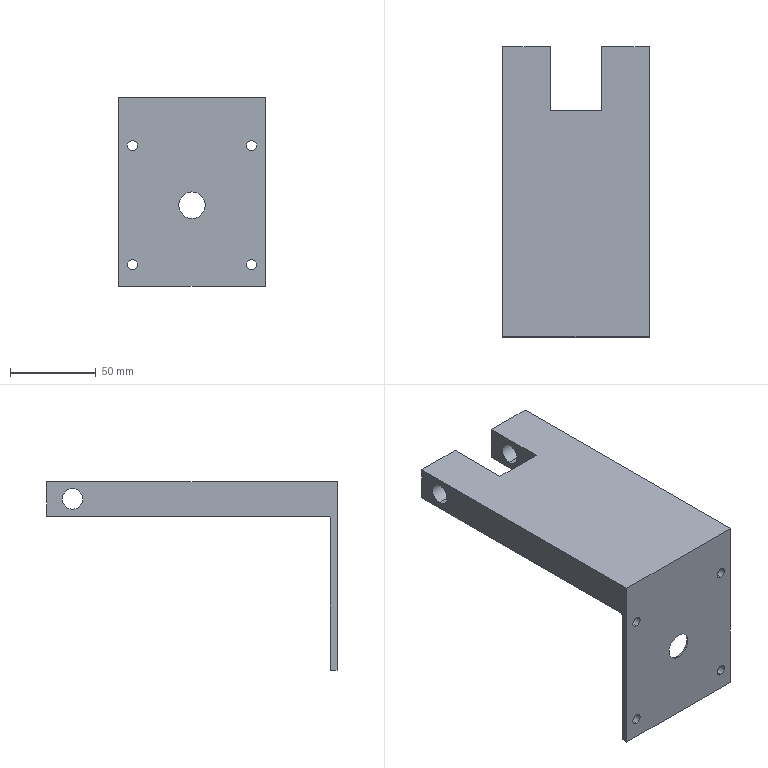Part | SolidWorks | features ICE 7, Cut 2, Extrusion 1, Fillet 1 | 1 solid | 33 faces | box 85.5 x 169.57 x 110 mm | volume 284547 mm3 | cylinder 19 | plane 14 | commonest cylinder face diameters 6 x8 12 x4 15.5 x2 20 x2 75 x2 2 x1
STEP:
#1=CARTESIAN_POINT('',(0.,-39.57,-52.75));
#2=VERTEX_POINT('',#1);
#3=CARTESIAN_POINT('',(0.,-39.57,-32.75));
#4=VERTEX_POINT('',#3);
#5=CARTESIAN_POINT('',(0.,-39.57,-42.75));
#6=DIRECTION('',(0.,1.,0.));
#7=DIRECTION('',(0.,0.,1.));
#8=AXIS2_PLACEMENT_3D('',#5,#6,#7);
#9=CIRCLE('',#8,10.);
#10=EDGE_CURVE('',#2,#4,#9,.T.);
#11=ORIENTED_EDGE('',*,*,#10,.F.);
#12=CARTESIAN_POINT('',(0.,-38.07,-52.75));
#13=VERTEX_POINT('',#12);
#14=CARTESIAN_POINT('',(0.,-39.57,-52.75));
#15=DIRECTION('',(0.,1.,0.));
#16=VECTOR('',#15,1000.);
#17=LINE('',#14,#16);
#18=EDGE_CURVE('',#2,#13,#17,.T.);
#19=ORIENTED_EDGE('',*,*,#18,.T.);
#20=CARTESIAN_POINT('',(0.,-38.07,-32.75));
#21=VERTEX_POINT('',#20);
#22=CARTESIAN_POINT('',(0.,-38.07,-42.75));
#23=DIRECTION('',(0.,1.,0.));
#24=DIRECTION('',(0.,0.,1.));
#25=AXIS2_PLACEMENT_3D('',#22,#23,#24);
#26=CIRCLE('',#25,10.);
#27=EDGE_CURVE('',#13,#21,#26,.T.);
#28=ORIENTED_EDGE('',*,*,#27,.T.);
#29=CARTESIAN_POINT('',(0.,-39.57,-32.75));
#30=DIRECTION('',(0.,1.,0.));
#31=VECTOR('',#30,1000.);
#32=LINE('',#29,#31);
#33=EDGE_CURVE('',#4,#21,#32,.T.);
#34=ORIENTED_EDGE('',*,*,#33,.F.);
#35=EDGE_LOOP('',(#11,#19,#28,#34));
#36=FACE_OUTER_BOUND('',#35,.T.);
#37=CARTESIAN_POINT('',(0.,-39.57,-42.75));
#38=DIRECTION('',(0.,1.,0.));
#39=DIRECTION('',(0.,0.,1.));
#40=AXIS2_PLACEMENT_3D('',#37,#38,#39);
#41=CYLINDRICAL_SURFACE('',#40,10.);
#42=ADVANCED_FACE('',(#36),#41,.F.);
#43=CARTESIAN_POINT('',(0.,-38.07,-80.25));
#44=VERTEX_POINT('',#43);
#45=CARTESIAN_POINT('',(0.,-38.07,-5.25));
#46=VERTEX_POINT('',#45);
#47=CARTESIAN_POINT('',(0.,-38.07,-42.75));
#48=DIRECTION('',(0.,1.,0.));
#49=DIRECTION('',(0.,0.,1.));
#50=AXIS2_PLACEMENT_3D('',#47,#48,#49);
#51=CIRCLE('',#50,37.5);
#52=EDGE_CURVE('',#44,#46,#51,.T.);
#53=ORIENTED_EDGE('',*,*,#52,.F.);
#54=CARTESIAN_POINT('',(0.,-36.57,-80.25));
#55=VERTEX_POINT('',#54);
#56=CARTESIAN_POINT('',(0.,-38.07,-80.25));
#57=DIRECTION('',(0.,1.,0.));
#58=VECTOR('',#57,1000.);
#59=LINE('',#56,#58);
#60=EDGE_CURVE('',#44,#55,#59,.T.);
#61=ORIENTED_EDGE('',*,*,#60,.T.);
#62=CARTESIAN_POINT('',(0.,-36.57,-5.25));
#63=VERTEX_POINT('',#62);
#64=CARTESIAN_POINT('',(0.,-36.57,-42.75));
#65=DIRECTION('',(0.,1.,0.));
#66=DIRECTION('',(0.,0.,1.));
#67=AXIS2_PLACEMENT_3D('',#64,#65,#66);
#68=CIRCLE('',#67,37.5);
#69=EDGE_CURVE('',#55,#63,#68,.T.);
#70=ORIENTED_EDGE('',*,*,#69,.T.);
#71=CARTESIAN_POINT('',(0.,-38.07,-5.25));
#72=DIRECTION('',(0.,1.,0.));
#73=VECTOR('',#72,1000.);
#74=LINE('',#71,#73);
#75=EDGE_CURVE('',#46,#63,#74,.T.);
#76=ORIENTED_EDGE('',*,*,#75,.F.);
#77=EDGE_LOOP('',(#53,#61,#70,#76));
#78=FACE_OUTER_BOUND('',#77,.T.);
#79=CARTESIAN_POINT('',(0.,-38.07,-42.75));
#80=DIRECTION('',(0.,1.,0.));
#81=DIRECTION('',(0.,0.,1.));
#82=AXIS2_PLACEMENT_3D('',#79,#80,#81);
#83=CYLINDRICAL_SURFACE('',#82,37.5);
#84=ADVANCED_FACE('',(#78),#83,.F.);
#85=CARTESIAN_POINT('',(34.8,-40.57,-74.55));
#86=VERTEX_POINT('',#85);
#87=CARTESIAN_POINT('',(34.8,-40.57,-80.55));
#88=VERTEX_POINT('',#87);
#89=CARTESIAN_POINT('',(34.8,-40.57,-77.55));
#90=DIRECTION('',(0.,-1.,0.));
#91=DIRECTION('',(0.,0.,-1.));
#92=AXIS2_PLACEMENT_3D('',#89,#90,#91);
#93=CIRCLE('',#92,3.);
#94=EDGE_CURVE('',#86,#88,#93,.T.);
#95=ORIENTED_EDGE('',*,*,#94,.T.);
#96=CARTESIAN_POINT('',(34.8,-36.57,-80.55));
#97=VERTEX_POINT('',#96);
#98=CARTESIAN_POINT('',(34.8,-126.57,-80.55));
#99=DIRECTION('',(0.,1.,0.));
#100=VECTOR('',#99,1000.);
#101=LINE('',#98,#100);
#102=EDGE_CURVE('',#88,#97,#101,.T.);
#103=ORIENTED_EDGE('',*,*,#102,.T.);
#104=CARTESIAN_POINT('',(34.8,-36.57,-74.55));
#105=VERTEX_POINT('',#104);
#106=CARTESIAN_POINT('',(34.8,-36.57,-77.55));
#107=DIRECTION('',(0.,1.,0.));
#108=DIRECTION('',(0.,0.,1.));
#109=AXIS2_PLACEMENT_3D('',#106,#107,#108);
#110=CIRCLE('',#109,3.);
#111=EDGE_CURVE('',#97,#105,#110,.T.);
#112=ORIENTED_EDGE('',*,*,#111,.T.);
#113=CARTESIAN_POINT('',(34.8,-126.57,-74.55));
#114=DIRECTION('',(0.,1.,0.));
#115=VECTOR('',#114,1000.);
#116=LINE('',#113,#115);
#117=EDGE_CURVE('',#86,#105,#116,.T.);
#118=ORIENTED_EDGE('',*,*,#117,.F.);
#119=EDGE_LOOP('',(#95,#103,#112,#118));
#120=FACE_OUTER_BOUND('',#119,.T.);
#121=CARTESIAN_POINT('',(34.8,-126.57,-77.55));
#122=DIRECTION('',(0.,1.,0.));
#123=DIRECTION('',(0.,0.,1.));
#124=AXIS2_PLACEMENT_3D('',#121,#122,#123);
#125=CYLINDRICAL_SURFACE('',#124,3.);
#126=ADVANCED_FACE('',(#120),#125,.F.);
#127=CARTESIAN_POINT('',(-34.8,-40.57,-4.95));
#128=VERTEX_POINT('',#127);
#129=CARTESIAN_POINT('',(-34.8,-40.57,-10.95));
#130=VERTEX_POINT('',#129);
#131=CARTESIAN_POINT('',(-34.8,-40.57,-7.95));
#132=DIRECTION('',(0.,-1.,0.));
#133=DIRECTION('',(0.,0.,-1.));
#134=AXIS2_PLACEMENT_3D('',#131,#132,#133);
#135=CIRCLE('',#134,3.);
#136=EDGE_CURVE('',#128,#130,#135,.T.);
#137=ORIENTED_EDGE('',*,*,#136,.T.);
#138=CARTESIAN_POINT('',(-34.8,-36.57,-10.95));
#139=VERTEX_POINT('',#138);
#140=CARTESIAN_POINT('',(-34.8,-126.57,-10.95));
#141=DIRECTION('',(0.,1.,0.));
#142=VECTOR('',#141,1000.);
#143=LINE('',#140,#142);
#144=EDGE_CURVE('',#130,#139,#143,.T.);
#145=ORIENTED_EDGE('',*,*,#144,.T.);
#146=CARTESIAN_POINT('',(-34.8,-36.57,-4.95));
#147=VERTEX_POINT('',#146);
#148=CARTESIAN_POINT('',(-34.8,-36.57,-7.95));
#149=DIRECTION('',(0.,1.,0.));
#150=DIRECTION('',(0.,0.,1.));
#151=AXIS2_PLACEMENT_3D('',#148,#149,#150);
#152=CIRCLE('',#151,3.);
#153=EDGE_CURVE('',#139,#147,#152,.T.);
#154=ORIENTED_EDGE('',*,*,#153,.T.);
#155=CARTESIAN_POINT('',(-34.8,-126.57,-4.95));
#156=DIRECTION('',(0.,1.,0.));
#157=VECTOR('',#156,1000.);
#158=LINE('',#155,#157);
#159=EDGE_CURVE('',#128,#147,#158,.T.);
#160=ORIENTED_EDGE('',*,*,#159,.F.);
#161=EDGE_LOOP('',(#137,#145,#154,#160));
#162=FACE_OUTER_BOUND('',#161,.T.);
#163=CARTESIAN_POINT('',(-34.8,-126.57,-7.95));
#164=DIRECTION('',(0.,1.,0.));
#165=DIRECTION('',(0.,0.,1.));
#166=AXIS2_PLACEMENT_3D('',#163,#164,#165);
#167=CYLINDRICAL_SURFACE('',#166,3.);
#168=ADVANCED_FACE('',(#162),#167,.F.);
#169=CARTESIAN_POINT('',(34.8,-40.57,-4.95));
#170=VERTEX_POINT('',#169);
#171=CARTESIAN_POINT('',(34.8,-40.57,-10.95));
#172=VERTEX_POINT('',#171);
#173=CARTESIAN_POINT('',(34.8,-40.57,-7.95));
#174=DIRECTION('',(0.,-1.,0.));
#175=DIRECTION('',(0.,0.,-1.));
#176=AXIS2_PLACEMENT_3D('',#173,#174,#175);
#177=CIRCLE('',#176,3.);
#178=EDGE_CURVE('',#170,#172,#177,.T.);
#179=ORIENTED_EDGE('',*,*,#178,.T.);
#180=CARTESIAN_POINT('',(34.8,-36.57,-10.95));
#181=VERTEX_POINT('',#180);
#182=CARTESIAN_POINT('',(34.8,-126.57,-10.95));
#183=DIRECTION('',(0.,1.,0.));
#184=VECTOR('',#183,1000.);
#185=LINE('',#182,#184);
#186=EDGE_CURVE('',#172,#181,#185,.T.);
#187=ORIENTED_EDGE('',*,*,#186,.T.);
#188=CARTESIAN_POINT('',(34.8,-36.57,-4.95));
#189=VERTEX_POINT('',#188);
#190=CARTESIAN_POINT('',(34.8,-36.57,-7.95));
#191=DIRECTION('',(0.,1.,0.));
#192=DIRECTION('',(0.,0.,1.));
#193=AXIS2_PLACEMENT_3D('',#190,#191,#192);
#194=CIRCLE('',#193,3.);
#195=EDGE_CURVE('',#181,#189,#194,.T.);
#196=ORIENTED_EDGE('',*,*,#195,.T.);
#197=CARTESIAN_POINT('',(34.8,-126.57,-4.95));
#198=DIRECTION('',(0.,1.,0.));
#199=VECTOR('',#198,1000.);
#200=LINE('',#197,#199);
#201=EDGE_CURVE('',#170,#189,#200,.T.);
#202=ORIENTED_EDGE('',*,*,#201,.F.);
#203=EDGE_LOOP('',(#179,#187,#196,#202));
#204=FACE_OUTER_BOUND('',#203,.T.);
#205=CARTESIAN_POINT('',(34.8,-126.57,-7.95));
#206=DIRECTION('',(0.,1.,0.));
#207=DIRECTION('',(0.,0.,1.));
#208=AXIS2_PLACEMENT_3D('',#205,#206,#207);
#209=CYLINDRICAL_SURFACE('',#208,3.);
#210=ADVANCED_FACE('',(#204),#209,.F.);
#211=CARTESIAN_POINT('',(-34.8,-40.57,-74.55));
#212=VERTEX_POINT('',#211);
#213=CARTESIAN_POINT('',(-34.8,-40.57,-80.55));
#214=VERTEX_POINT('',#213);
#215=CARTESIAN_POINT('',(-34.8,-40.57,-77.55));
#216=DIRECTION('',(0.,-1.,0.));
#217=DIRECTION('',(0.,0.,-1.));
#218=AXIS2_PLACEMENT_3D('',#215,#216,#217);
#219=CIRCLE('',#218,3.);
#220=EDGE_CURVE('',#212,#214,#219,.T.);
#221=ORIENTED_EDGE('',*,*,#220,.T.);
#222=CARTESIAN_POINT('',(-34.8,-36.57,-80.55));
#223=VERTEX_POINT('',#222);
#224=CARTESIAN_POINT('',(-34.8,-126.57,-80.55));
#225=DIRECTION('',(0.,1.,0.));
#226=VECTOR('',#225,1000.);
#227=LINE('',#224,#226);
#228=EDGE_CURVE('',#214,#223,#227,.T.);
#229=ORIENTED_EDGE('',*,*,#228,.T.);
#230=CARTESIAN_POINT('',(-34.8,-36.57,-74.55));
#231=VERTEX_POINT('',#230);
#232=CARTESIAN_POINT('',(-34.8,-36.57,-77.55));
#233=DIRECTION('',(0.,1.,0.));
#234=DIRECTION('',(0.,0.,1.));
#235=AXIS2_PLACEMENT_3D('',#232,#233,#234);
#236=CIRCLE('',#235,3.);
#237=EDGE_CURVE('',#223,#231,#236,.T.);
#238=ORIENTED_EDGE('',*,*,#237,.T.);
#239=CARTESIAN_POINT('',(-34.8,-126.57,-74.55));
#240=DIRECTION('',(0.,1.,0.));
#241=VECTOR('',#240,1000.);
#242=LINE('',#239,#241);
#243=EDGE_CURVE('',#212,#231,#242,.T.);
#244=ORIENTED_EDGE('',*,*,#243,.F.);
#245=EDGE_LOOP('',(#221,#229,#238,#244));
#246=FACE_OUTER_BOUND('',#245,.T.);
#247=CARTESIAN_POINT('',(-34.8,-126.57,-77.55));
#248=DIRECTION('',(0.,1.,0.));
#249=DIRECTION('',(0.,0.,1.));
#250=AXIS2_PLACEMENT_3D('',#247,#248,#249);
#251=CYLINDRICAL_SURFACE('',#250,3.);
#252=ADVANCED_FACE('',(#246),#251,.F.);
#253=CARTESIAN_POINT('',(-15.052,114.,4.));
#254=VERTEX_POINT('',#253);
#255=CARTESIAN_POINT('',(-15.052,114.,16.));
#256=VERTEX_POINT('',#255);
#257=CARTESIAN_POINT('',(-15.052,114.,10.));
#258=DIRECTION('',(-1.,0.,0.));
#259=DIRECTION('',(0.,0.,1.));
#260=AXIS2_PLACEMENT_3D('',#257,#258,#259);
#261=CIRCLE('',#260,6.);
#262=EDGE_CURVE('',#254,#256,#261,.T.);
#263=ORIENTED_EDGE('',*,*,#262,.F.);
#264=CARTESIAN_POINT('',(-42.75,114.,4.));
#265=VERTEX_POINT('',#264);
#266=CARTESIAN_POINT('',(42.75,114.,4.));
#267=DIRECTION('',(-1.,0.,0.));
#268=VECTOR('',#267,1000.);
#269=LINE('',#266,#268);
#270=EDGE_CURVE('',#254,#265,#269,.T.);
#271=ORIENTED_EDGE('',*,*,#270,.T.);
#272=CARTESIAN_POINT('',(-42.75,114.,16.));
#273=VERTEX_POINT('',#272);
#274=CARTESIAN_POINT('',(-42.75,114.,10.));
#275=DIRECTION('',(1.,0.,0.));
#276=DIRECTION('',(0.,0.,-1.));
#277=AXIS2_PLACEMENT_3D('',#274,#275,#276);
#278=CIRCLE('',#277,6.);
#279=EDGE_CURVE('',#273,#265,#278,.T.);
#280=ORIENTED_EDGE('',*,*,#279,.F.);
#281=CARTESIAN_POINT('',(42.75,114.,16.));
#282=DIRECTION('',(-1.,0.,0.));
#283=VECTOR('',#282,1000.);
#284=LINE('',#281,#283);
#285=EDGE_CURVE('',#256,#273,#284,.T.);
#286=ORIENTED_EDGE('',*,*,#285,.F.);
#287=EDGE_LOOP('',(#263,#271,#280,#286));
#288=FACE_OUTER_BOUND('',#287,.T.);
#289=CARTESIAN_POINT('',(42.75,114.,10.));
#290=DIRECTION('',(-1.,0.,0.));
#291=DIRECTION('',(0.,0.,1.));
#292=AXIS2_PLACEMENT_3D('',#289,#290,#291);
#293=CYLINDRICAL_SURFACE('',#292,6.);
#294=ADVANCED_FACE('',(#288),#293,.F.);
#295=CARTESIAN_POINT('',(42.75,114.,4.));
#296=VERTEX_POINT('',#295);
#297=CARTESIAN_POINT('',(42.75,114.,16.));
#298=VERTEX_POINT('',#297);
#299=CARTESIAN_POINT('',(42.75,114.,10.));
#300=DIRECTION('',(-1.,0.,0.));
#301=DIRECTION('',(0.,0.,1.));
#302=AXIS2_PLACEMENT_3D('',#299,#300,#301);
#303=CIRCLE('',#302,6.);
#304=EDGE_CURVE('',#296,#298,#303,.T.);
#305=ORIENTED_EDGE('',*,*,#304,.F.);
#306=CARTESIAN_POINT('',(14.948,114.,4.));
#307=VERTEX_POINT('',#306);
#308=CARTESIAN_POINT('',(42.75,114.,4.));
#309=DIRECTION('',(-1.,0.,0.));
#310=VECTOR('',#309,1000.);
#311=LINE('',#308,#310);
#312=EDGE_CURVE('',#296,#307,#311,.T.);
#313=ORIENTED_EDGE('',*,*,#312,.T.);
#314=CARTESIAN_POINT('',(14.948,114.,16.));
#315=VERTEX_POINT('',#314);
#316=CARTESIAN_POINT('',(14.948,114.,10.));
#317=DIRECTION('',(1.,0.,0.));
#318=DIRECTION('',(0.,1.,0.));
#319=AXIS2_PLACEMENT_3D('',#316,#317,#318);
#320=CIRCLE('',#319,6.);
#321=EDGE_CURVE('',#315,#307,#320,.T.);
#322=ORIENTED_EDGE('',*,*,#321,.F.);
#323=CARTESIAN_POINT('',(42.75,114.,16.));
#324=DIRECTION('',(-1.,0.,0.));
#325=VECTOR('',#324,1000.);
#326=LINE('',#323,#325);
#327=EDGE_CURVE('',#298,#315,#326,.T.);
#328=ORIENTED_EDGE('',*,*,#327,.F.);
#329=EDGE_LOOP('',(#305,#313,#322,#328));
#330=FACE_OUTER_BOUND('',#329,.T.);
#331=CARTESIAN_POINT('',(42.75,114.,10.));
#332=DIRECTION('',(-1.,0.,0.));
#333=DIRECTION('',(0.,0.,1.));
#334=AXIS2_PLACEMENT_3D('',#331,#332,#333);
#335=CYLINDRICAL_SURFACE('',#334,6.);
#336=ADVANCED_FACE('',(#330),#335,.F.);
#337=CARTESIAN_POINT('',(0.,-40.57,-50.5));
#338=VERTEX_POINT('',#337);
#339=CARTESIAN_POINT('',(0.,-40.57,-35.));
#340=VERTEX_POINT('',#339);
#341=CARTESIAN_POINT('',(0.,-40.57,-42.75));
#342=DIRECTION('',(0.,1.,0.));
#343=DIRECTION('',(0.,0.,1.));
#344=AXIS2_PLACEMENT_3D('',#341,#342,#343);
#345=CIRCLE('',#344,7.75);
#346=EDGE_CURVE('',#338,#340,#345,.T.);
#347=ORIENTED_EDGE('',*,*,#346,.F.);
#348=CARTESIAN_POINT('',(0.,-39.57,-50.5));
#349=VERTEX_POINT('',#348);
#350=CARTESIAN_POINT('',(0.,-40.57,-50.5));
#351=DIRECTION('',(0.,1.,0.));
#352=VECTOR('',#351,1000.);
#353=LINE('',#350,#352);
#354=EDGE_CURVE('',#338,#349,#353,.T.);
#355=ORIENTED_EDGE('',*,*,#354,.T.);
#356=CARTESIAN_POINT('',(0.,-39.57,-35.));
#357=VERTEX_POINT('',#356);
#358=CARTESIAN_POINT('',(0.,-39.57,-42.75));
#359=DIRECTION('',(0.,-1.,0.));
#360=DIRECTION('',(0.,0.,1.));
#361=AXIS2_PLACEMENT_3D('',#358,#359,#360);
#362=CIRCLE('',#361,7.75);
#363=EDGE_CURVE('',#357,#349,#362,.T.);
#364=ORIENTED_EDGE('',*,*,#363,.F.);
#365=CARTESIAN_POINT('',(0.,-40.57,-35.));
#366=DIRECTION('',(0.,1.,0.));
#367=VECTOR('',#366,1000.);
#368=LINE('',#365,#367);
#369=EDGE_CURVE('',#340,#357,#368,.T.);
#370=ORIENTED_EDGE('',*,*,#369,.F.);
#371=EDGE_LOOP('',(#347,#355,#364,#370));
#372=FACE_OUTER_BOUND('',#371,.T.);
#373=CARTESIAN_POINT('',(0.,-40.57,-42.75));
#374=DIRECTION('',(0.,1.,0.));
#375=DIRECTION('',(0.,0.,1.));
#376=AXIS2_PLACEMENT_3D('',#373,#374,#375);
#377=CYLINDRICAL_SURFACE('',#376,7.75);
#378=ADVANCED_FACE('',(#372),#377,.F.);
#379=ORIENTED_EDGE('',*,*,#354,.F.);
#380=CARTESIAN_POINT('',(0.,-40.57,-42.75));
#381=DIRECTION('',(0.,1.,0.));
#382=DIRECTION('',(0.,0.,1.));
#383=AXIS2_PLACEMENT_3D('',#380,#381,#382);
#384=CIRCLE('',#383,7.75);
#385=EDGE_CURVE('',#340,#338,#384,.T.);
#386=ORIENTED_EDGE('',*,*,#385,.F.);
#387=ORIENTED_EDGE('',*,*,#369,.T.);
#388=CARTESIAN_POINT('',(0.,-39.57,-42.75));
#389=DIRECTION('',(0.,-1.,0.));
#390=DIRECTION('',(0.,0.,1.));
#391=AXIS2_PLACEMENT_3D('',#388,#389,#390);
#392=CIRCLE('',#391,7.75);
#393=EDGE_CURVE('',#349,#357,#392,.T.);
#394=ORIENTED_EDGE('',*,*,#393,.F.);
#395=EDGE_LOOP('',(#379,#386,#387,#394));
#396=FACE_OUTER_BOUND('',#395,.T.);
#397=CARTESIAN_POINT('',(0.,-40.57,-42.75));
#398=DIRECTION('',(0.,1.,0.));
#399=DIRECTION('',(0.,0.,1.));
#400=AXIS2_PLACEMENT_3D('',#397,#398,#399);
#401=CYLINDRICAL_SURFACE('',#400,7.75);
#402=ADVANCED_FACE('',(#396),#401,.F.);
#403=ORIENTED_EDGE('',*,*,#279,.T.);
#404=CARTESIAN_POINT('',(-42.75,114.,10.));
#405=DIRECTION('',(1.,0.,0.));
#406=DIRECTION('',(0.,0.,-1.));
#407=AXIS2_PLACEMENT_3D('',#404,#405,#406);
#408=CIRCLE('',#407,6.);
#409=EDGE_CURVE('',#265,#273,#408,.T.);
#410=ORIENTED_EDGE('',*,*,#409,.T.);
#411=EDGE_LOOP('',(#403,#410));
#412=FACE_BOUND('',#411,.T.);
#413=CARTESIAN_POINT('',(-42.75,-40.57,20.));
#414=VERTEX_POINT('',#413);
#415=CARTESIAN_POINT('',(-42.75,-40.57,-90.));
#416=VERTEX_POINT('',#415);
#417=CARTESIAN_POINT('',(-42.75,-40.57,20.));
#418=DIRECTION('',(0.,0.,-1.));
#419=VECTOR('',#418,1000.);
#420=LINE('',#417,#419);
#421=EDGE_CURVE('',#414,#416,#420,.T.);
#422=ORIENTED_EDGE('',*,*,#421,.F.);
#423=CARTESIAN_POINT('',(-42.75,129.,20.));
#424=VERTEX_POINT('',#423);
#425=CARTESIAN_POINT('',(-42.75,59.,20.));
#426=DIRECTION('',(0.,-1.,0.));
#427=VECTOR('',#426,1000.);
#428=LINE('',#425,#427);
#429=EDGE_CURVE('',#424,#414,#428,.T.);
#430=ORIENTED_EDGE('',*,*,#429,.F.);
#431=CARTESIAN_POINT('',(-42.75,129.,0.));
#432=VERTEX_POINT('',#431);
#433=CARTESIAN_POINT('',(-42.75,129.,20.));
#434=DIRECTION('',(0.,0.,-1.));
#435=VECTOR('',#434,1000.);
#436=LINE('',#433,#435);
#437=EDGE_CURVE('',#424,#432,#436,.T.);
#438=ORIENTED_EDGE('',*,*,#437,.T.);
#439=CARTESIAN_POINT('',(-42.75,-35.57,0.));
#440=VERTEX_POINT('',#439);
#441=CARTESIAN_POINT('',(-42.75,-59.,0.));
#442=DIRECTION('',(0.,-1.,0.));
#443=VECTOR('',#442,1000.);
#444=LINE('',#441,#443);
#445=EDGE_CURVE('',#432,#440,#444,.T.);
#446=ORIENTED_EDGE('',*,*,#445,.T.);
#447=CARTESIAN_POINT('',(-42.75,-36.57,-1.));
#448=VERTEX_POINT('',#447);
#449=CARTESIAN_POINT('',(-42.75,-35.57,-1.));
#450=DIRECTION('',(1.,0.,0.));
#451=DIRECTION('',(0.,0.,-1.));
#452=AXIS2_PLACEMENT_3D('',#449,#450,#451);
#453=CIRCLE('',#452,1.);
#454=EDGE_CURVE('',#440,#448,#453,.T.);
#455=ORIENTED_EDGE('',*,*,#454,.T.);
#456=CARTESIAN_POINT('',(-42.75,-36.57,-90.));
#457=VERTEX_POINT('',#456);
#458=CARTESIAN_POINT('',(-42.75,-36.57,-90.));
#459=DIRECTION('',(0.,0.,1.));
#460=VECTOR('',#459,1000.);
#461=LINE('',#458,#460);
#462=EDGE_CURVE('',#457,#448,#461,.T.);
#463=ORIENTED_EDGE('',*,*,#462,.F.);
#464=CARTESIAN_POINT('',(-42.75,0.,-90.));
#465=DIRECTION('',(0.,-1.,0.));
#466=VECTOR('',#465,1000.);
#467=LINE('',#464,#466);
#468=EDGE_CURVE('',#457,#416,#467,.T.);
#469=ORIENTED_EDGE('',*,*,#468,.T.);
#470=EDGE_LOOP('',(#422,#430,#438,#446,#455,#463,#469));
#471=FACE_OUTER_BOUND('',#470,.T.);
#472=CARTESIAN_POINT('',(-42.75,-59.,20.));
#473=DIRECTION('',(1.,0.,0.));
#474=DIRECTION('',(0.,0.,-1.));
#475=AXIS2_PLACEMENT_3D('',#472,#473,#474);
#476=PLANE('',#475);
#477=ADVANCED_FACE('',(#412,#471),#476,.F.);
#478=CARTESIAN_POINT('',(42.75,114.,10.));
#479=DIRECTION('',(-1.,0.,0.));
#480=DIRECTION('',(0.,0.,1.));
#481=AXIS2_PLACEMENT_3D('',#478,#479,#480);
#482=CIRCLE('',#481,6.);
#483=EDGE_CURVE('',#298,#296,#482,.T.);
#484=ORIENTED_EDGE('',*,*,#483,.T.);
#485=ORIENTED_EDGE('',*,*,#304,.T.);
#486=EDGE_LOOP('',(#484,#485));
#487=FACE_BOUND('',#486,.T.);
#488=CARTESIAN_POINT('',(42.75,-40.57,-90.));
#489=VERTEX_POINT('',#488);
#490=CARTESIAN_POINT('',(42.75,-40.57,20.));
#491=VERTEX_POINT('',#490);
#492=CARTESIAN_POINT('',(42.75,-40.57,0.));
#493=DIRECTION('',(0.,0.,1.));
#494=VECTOR('',#493,1000.);
#495=LINE('',#492,#494);
#496=EDGE_CURVE('',#489,#491,#495,.T.);
#497=ORIENTED_EDGE('',*,*,#496,.F.);
#498=CARTESIAN_POINT('',(42.75,-36.57,-90.));
#499=VERTEX_POINT('',#498);
#500=CARTESIAN_POINT('',(42.75,0.,-90.));
#501=DIRECTION('',(0.,1.,0.));
#502=VECTOR('',#501,1000.);
#503=LINE('',#500,#502);
#504=EDGE_CURVE('',#489,#499,#503,.T.);
#505=ORIENTED_EDGE('',*,*,#504,.T.);
#506=CARTESIAN_POINT('',(42.75,-36.57,-1.));
#507=VERTEX_POINT('',#506);
#508=CARTESIAN_POINT('',(42.75,-36.57,-90.));
#509=DIRECTION('',(0.,0.,1.));
#510=VECTOR('',#509,1000.);
#511=LINE('',#508,#510);
#512=EDGE_CURVE('',#499,#507,#511,.T.);
#513=ORIENTED_EDGE('',*,*,#512,.T.);
#514=CARTESIAN_POINT('',(42.75,-35.57,0.));
#515=VERTEX_POINT('',#514);
#516=CARTESIAN_POINT('',(42.75,-35.57,-1.));
#517=DIRECTION('',(-1.,0.,0.));
#518=DIRECTION('',(0.,-1.,0.));
#519=AXIS2_PLACEMENT_3D('',#516,#517,#518);
#520=CIRCLE('',#519,1.);
#521=EDGE_CURVE('',#507,#515,#520,.T.);
#522=ORIENTED_EDGE('',*,*,#521,.T.);
#523=CARTESIAN_POINT('',(42.75,129.,0.));
#524=VERTEX_POINT('',#523);
#525=CARTESIAN_POINT('',(42.75,-59.,0.));
#526=DIRECTION('',(0.,1.,0.));
#527=VECTOR('',#526,1000.);
#528=LINE('',#525,#527);
#529=EDGE_CURVE('',#515,#524,#528,.T.);
#530=ORIENTED_EDGE('',*,*,#529,.T.);
#531=CARTESIAN_POINT('',(42.75,129.,20.));
#532=VERTEX_POINT('',#531);
#533=CARTESIAN_POINT('',(42.75,129.,20.));
#534=DIRECTION('',(0.,0.,-1.));
#535=VECTOR('',#534,1000.);
#536=LINE('',#533,#535);
#537=EDGE_CURVE('',#532,#524,#536,.T.);
#538=ORIENTED_EDGE('',*,*,#537,.F.);
#539=CARTESIAN_POINT('',(42.75,129.,20.));
#540=DIRECTION('',(0.,1.,0.));
#541=VECTOR('',#540,1000.);
#542=LINE('',#539,#541);
#543=EDGE_CURVE('',#491,#532,#542,.T.);
#544=ORIENTED_EDGE('',*,*,#543,.F.);
#545=EDGE_LOOP('',(#497,#505,#513,#522,#530,#538,#544));
#546=FACE_OUTER_BOUND('',#545,.T.);
#547=CARTESIAN_POINT('',(42.75,-59.,20.));
#548=DIRECTION('',(-1.,0.,0.));
#549=DIRECTION('',(0.,-1.,0.));
#550=AXIS2_PLACEMENT_3D('',#547,#548,#549);
#551=PLANE('',#550);
#552=ADVANCED_FACE('',(#487,#546),#551,.F.);
#553=ORIENTED_EDGE('',*,*,#429,.T.);
#554=CARTESIAN_POINT('',(42.75,-40.57,20.));
#555=DIRECTION('',(-1.,0.,0.));
#556=VECTOR('',#555,1000.);
#557=LINE('',#554,#556);
#558=EDGE_CURVE('',#491,#414,#557,.T.);
#559=ORIENTED_EDGE('',*,*,#558,.F.);
#560=ORIENTED_EDGE('',*,*,#543,.T.);
#561=CARTESIAN_POINT('',(14.948,129.,20.));
#562=VERTEX_POINT('',#561);
#563=CARTESIAN_POINT('',(-42.75,129.,20.));
#564=DIRECTION('',(-1.,0.,0.));
#565=VECTOR('',#564,1000.);
#566=LINE('',#563,#565);
#567=EDGE_CURVE('',#532,#562,#566,.T.);
#568=ORIENTED_EDGE('',*,*,#567,.T.);
#569=CARTESIAN_POINT('',(14.948,92.,20.));
#570=VERTEX_POINT('',#569);
#571=CARTESIAN_POINT('',(14.948,129.,20.));
#572=DIRECTION('',(0.,1.,0.));
#573=VECTOR('',#572,1000.);
#574=LINE('',#571,#573);
#575=EDGE_CURVE('',#570,#562,#574,.T.);
#576=ORIENTED_EDGE('',*,*,#575,.F.);
#577=CARTESIAN_POINT('',(-15.052,92.,20.));
#578=VERTEX_POINT('',#577);
#579=CARTESIAN_POINT('',(-15.052,92.,20.));
#580=DIRECTION('',(1.,0.,0.));
#581=VECTOR('',#580,1000.);
#582=LINE('',#579,#581);
#583=EDGE_CURVE('',#578,#570,#582,.T.);
#584=ORIENTED_EDGE('',*,*,#583,.F.);
#585=CARTESIAN_POINT('',(-15.052,129.,20.));
#586=VERTEX_POINT('',#585);
#587=CARTESIAN_POINT('',(-15.052,92.,20.));
#588=DIRECTION('',(0.,-1.,0.));
#589=VECTOR('',#588,1000.);
#590=LINE('',#587,#589);
#591=EDGE_CURVE('',#586,#578,#590,.T.);
#592=ORIENTED_EDGE('',*,*,#591,.F.);
#593=CARTESIAN_POINT('',(-42.75,129.,20.));
#594=DIRECTION('',(-1.,0.,0.));
#595=VECTOR('',#594,1000.);
#596=LINE('',#593,#595);
#597=EDGE_CURVE('',#586,#424,#596,.T.);
#598=ORIENTED_EDGE('',*,*,#597,.T.);
#599=EDGE_LOOP('',(#553,#559,#560,#568,#576,#584,#592,#598));
#600=FACE_OUTER_BOUND('',#599,.T.);
#601=CARTESIAN_POINT('',(0.,0.,20.));
#602=DIRECTION('',(0.,0.,1.));
#603=DIRECTION('',(1.,0.,0.));
#604=AXIS2_PLACEMENT_3D('',#601,#602,#603);
#605=PLANE('',#604);
#606=ADVANCED_FACE('',(#600),#605,.T.);
#607=ORIENTED_EDGE('',*,*,#529,.F.);
#608=CARTESIAN_POINT('',(0.,-35.57,0.));
#609=DIRECTION('',(-1.,0.,0.));
#610=VECTOR('',#609,1000.);
#611=LINE('',#608,#610);
#612=EDGE_CURVE('',#515,#440,#611,.T.);
#613=ORIENTED_EDGE('',*,*,#612,.T.);
#614=ORIENTED_EDGE('',*,*,#445,.F.);
#615=CARTESIAN_POINT('',(-15.052,129.,0.));
#616=VERTEX_POINT('',#615);
#617=CARTESIAN_POINT('',(-42.75,129.,0.));
#618=DIRECTION('',(-1.,0.,0.));
#619=VECTOR('',#618,1000.);
#620=LINE('',#617,#619);
#621=EDGE_CURVE('',#616,#432,#620,.T.);
#622=ORIENTED_EDGE('',*,*,#621,.F.);
#623=CARTESIAN_POINT('',(-15.052,92.,0.));
#624=VERTEX_POINT('',#623);
#625=CARTESIAN_POINT('',(-15.052,92.,0.));
#626=DIRECTION('',(0.,-1.,0.));
#627=VECTOR('',#626,1000.);
#628=LINE('',#625,#627);
#629=EDGE_CURVE('',#616,#624,#628,.T.);
#630=ORIENTED_EDGE('',*,*,#629,.T.);
#631=CARTESIAN_POINT('',(14.948,92.,0.));
#632=VERTEX_POINT('',#631);
#633=CARTESIAN_POINT('',(-15.052,92.,0.));
#634=DIRECTION('',(1.,0.,0.));
#635=VECTOR('',#634,1000.);
#636=LINE('',#633,#635);
#637=EDGE_CURVE('',#624,#632,#636,.T.);
#638=ORIENTED_EDGE('',*,*,#637,.T.);
#639=CARTESIAN_POINT('',(14.948,129.,0.));
#640=VERTEX_POINT('',#639);
#641=CARTESIAN_POINT('',(14.948,129.,0.));
#642=DIRECTION('',(0.,1.,0.));
#643=VECTOR('',#642,1000.);
#644=LINE('',#641,#643);
#645=EDGE_CURVE('',#632,#640,#644,.T.);
#646=ORIENTED_EDGE('',*,*,#645,.T.);
#647=CARTESIAN_POINT('',(-42.75,129.,0.));
#648=DIRECTION('',(-1.,0.,0.));
#649=VECTOR('',#648,1000.);
#650=LINE('',#647,#649);
#651=EDGE_CURVE('',#524,#640,#650,.T.);
#652=ORIENTED_EDGE('',*,*,#651,.F.);
#653=EDGE_LOOP('',(#607,#613,#614,#622,#630,#638,#646,#652));
#654=FACE_OUTER_BOUND('',#653,.T.);
#655=CARTESIAN_POINT('',(0.,0.,0.));
#656=DIRECTION('',(0.,0.,1.));
#657=DIRECTION('',(1.,0.,0.));
#658=AXIS2_PLACEMENT_3D('',#655,#656,#657);
#659=PLANE('',#658);
#660=ADVANCED_FACE('',(#654),#659,.F.);
#661=ORIENTED_EDGE('',*,*,#597,.F.);
#662=CARTESIAN_POINT('',(-15.052,129.,0.));
#663=DIRECTION('',(0.,0.,1.));
#664=VECTOR('',#663,1000.);
#665=LINE('',#662,#664);
#666=EDGE_CURVE('',#616,#586,#665,.T.);
#667=ORIENTED_EDGE('',*,*,#666,.F.);
#668=ORIENTED_EDGE('',*,*,#621,.T.);
#669=ORIENTED_EDGE('',*,*,#437,.F.);
#670=EDGE_LOOP('',(#661,#667,#668,#669));
#671=FACE_OUTER_BOUND('',#670,.T.);
#672=CARTESIAN_POINT('',(-42.75,129.,20.));
#673=DIRECTION('',(0.,-1.,0.));
#674=DIRECTION('',(0.,0.,-1.));
#675=AXIS2_PLACEMENT_3D('',#672,#673,#674);
#676=PLANE('',#675);
#677=ADVANCED_FACE('',(#671),#676,.F.);
#678=ORIENTED_EDGE('',*,*,#651,.T.);
#679=CARTESIAN_POINT('',(14.948,129.,0.));
#680=DIRECTION('',(0.,0.,1.));
#681=VECTOR('',#680,1000.);
#682=LINE('',#679,#681);
#683=EDGE_CURVE('',#640,#562,#682,.T.);
#684=ORIENTED_EDGE('',*,*,#683,.T.);
#685=ORIENTED_EDGE('',*,*,#567,.F.);
#686=ORIENTED_EDGE('',*,*,#537,.T.);
#687=EDGE_LOOP('',(#678,#684,#685,#686));
#688=FACE_OUTER_BOUND('',#687,.T.);
#689=CARTESIAN_POINT('',(-42.75,129.,20.));
#690=DIRECTION('',(0.,-1.,0.));
#691=DIRECTION('',(0.,0.,-1.));
#692=AXIS2_PLACEMENT_3D('',#689,#690,#691);
#693=PLANE('',#692);
#694=ADVANCED_FACE('',(#688),#693,.F.);
#695=ORIENTED_EDGE('',*,*,#583,.T.);
#696=CARTESIAN_POINT('',(14.948,92.,0.));
#697=DIRECTION('',(0.,0.,1.));
#698=VECTOR('',#697,1000.);
#699=LINE('',#696,#698);
#700=EDGE_CURVE('',#632,#570,#699,.T.);
#701=ORIENTED_EDGE('',*,*,#700,.F.);
#702=ORIENTED_EDGE('',*,*,#637,.F.);
#703=CARTESIAN_POINT('',(-15.052,92.,0.));
#704=DIRECTION('',(0.,0.,1.));
#705=VECTOR('',#704,1000.);
#706=LINE('',#703,#705);
#707=EDGE_CURVE('',#624,#578,#706,.T.);
#708=ORIENTED_EDGE('',*,*,#707,.T.);
#709=EDGE_LOOP('',(#695,#701,#702,#708));
#710=FACE_OUTER_BOUND('',#709,.T.);
#711=CARTESIAN_POINT('',(-15.052,92.,0.));
#712=DIRECTION('',(0.,-1.,0.));
#713=DIRECTION('',(0.,0.,-1.));
#714=AXIS2_PLACEMENT_3D('',#711,#712,#713);
#715=PLANE('',#714);
#716=ADVANCED_FACE('',(#710),#715,.F.);
#717=CARTESIAN_POINT('',(-15.052,114.,10.));
#718=DIRECTION('',(-1.,0.,0.));
#719=DIRECTION('',(0.,0.,1.));
#720=AXIS2_PLACEMENT_3D('',#717,#718,#719);
#721=CIRCLE('',#720,6.);
#722=EDGE_CURVE('',#256,#254,#721,.T.);
#723=ORIENTED_EDGE('',*,*,#722,.T.);
#724=ORIENTED_EDGE('',*,*,#262,.T.);
#725=EDGE_LOOP('',(#723,#724));
#726=FACE_BOUND('',#725,.T.);
#727=ORIENTED_EDGE('',*,*,#591,.T.);
#728=ORIENTED_EDGE('',*,*,#707,.F.);
#729=ORIENTED_EDGE('',*,*,#629,.F.);
#730=ORIENTED_EDGE('',*,*,#666,.T.);
#731=EDGE_LOOP('',(#727,#728,#729,#730));
#732=FACE_OUTER_BOUND('',#731,.T.);
#733=CARTESIAN_POINT('',(-15.052,92.,0.));
#734=DIRECTION('',(-1.,0.,0.));
#735=DIRECTION('',(0.,0.,1.));
#736=AXIS2_PLACEMENT_3D('',#733,#734,#735);
#737=PLANE('',#736);
#738=ADVANCED_FACE('',(#726,#732),#737,.F.);
#739=ORIENTED_EDGE('',*,*,#321,.T.);
#740=CARTESIAN_POINT('',(14.948,114.,10.));
#741=DIRECTION('',(1.,0.,0.));
#742=DIRECTION('',(0.,1.,0.));
#743=AXIS2_PLACEMENT_3D('',#740,#741,#742);
#744=CIRCLE('',#743,6.);
#745=EDGE_CURVE('',#307,#315,#744,.T.);
#746=ORIENTED_EDGE('',*,*,#745,.T.);
#747=EDGE_LOOP('',(#739,#746));
#748=FACE_BOUND('',#747,.T.);
#749=ORIENTED_EDGE('',*,*,#575,.T.);
#750=ORIENTED_EDGE('',*,*,#683,.F.);
#751=ORIENTED_EDGE('',*,*,#645,.F.);
#752=ORIENTED_EDGE('',*,*,#700,.T.);
#753=EDGE_LOOP('',(#749,#750,#751,#752));
#754=FACE_OUTER_BOUND('',#753,.T.);
#755=CARTESIAN_POINT('',(14.948,129.,0.));
#756=DIRECTION('',(1.,0.,0.));
#757=DIRECTION('',(0.,1.,0.));
#758=AXIS2_PLACEMENT_3D('',#755,#756,#757);
#759=PLANE('',#758);
#760=ADVANCED_FACE('',(#748,#754),#759,.F.);
#761=ORIENTED_EDGE('',*,*,#312,.F.);
#762=ORIENTED_EDGE('',*,*,#483,.F.);
#763=ORIENTED_EDGE('',*,*,#327,.T.);
#764=ORIENTED_EDGE('',*,*,#745,.F.);
#765=EDGE_LOOP('',(#761,#762,#763,#764));
#766=FACE_OUTER_BOUND('',#765,.T.);
#767=CARTESIAN_POINT('',(42.75,114.,10.));
#768=DIRECTION('',(-1.,0.,0.));
#769=DIRECTION('',(0.,0.,1.));
#770=AXIS2_PLACEMENT_3D('',#767,#768,#769);
#771=CYLINDRICAL_SURFACE('',#770,6.);
#772=ADVANCED_FACE('',(#766),#771,.F.);
#773=ORIENTED_EDGE('',*,*,#270,.F.);
#774=ORIENTED_EDGE('',*,*,#722,.F.);
#775=ORIENTED_EDGE('',*,*,#285,.T.);
#776=ORIENTED_EDGE('',*,*,#409,.F.);
#777=EDGE_LOOP('',(#773,#774,#775,#776));
#778=FACE_OUTER_BOUND('',#777,.T.);
#779=CARTESIAN_POINT('',(42.75,114.,10.));
#780=DIRECTION('',(-1.,0.,0.));
#781=DIRECTION('',(0.,0.,1.));
#782=AXIS2_PLACEMENT_3D('',#779,#780,#781);
#783=CYLINDRICAL_SURFACE('',#782,6.);
#784=ADVANCED_FACE('',(#778),#783,.F.);
#785=ORIENTED_EDGE('',*,*,#385,.T.);
#786=ORIENTED_EDGE('',*,*,#346,.T.);
#787=EDGE_LOOP('',(#785,#786));
#788=FACE_BOUND('',#787,.T.);
#789=ORIENTED_EDGE('',*,*,#94,.F.);
#790=CARTESIAN_POINT('',(34.8,-40.57,-77.55));
#791=DIRECTION('',(0.,-1.,0.));
#792=DIRECTION('',(0.,0.,-1.));
#793=AXIS2_PLACEMENT_3D('',#790,#791,#792);
#794=CIRCLE('',#793,3.);
#795=EDGE_CURVE('',#88,#86,#794,.T.);
#796=ORIENTED_EDGE('',*,*,#795,.F.);
#797=EDGE_LOOP('',(#789,#796));
#798=FACE_BOUND('',#797,.T.);
#799=ORIENTED_EDGE('',*,*,#136,.F.);
#800=CARTESIAN_POINT('',(-34.8,-40.57,-7.95));
#801=DIRECTION('',(0.,-1.,0.));
#802=DIRECTION('',(0.,0.,-1.));
#803=AXIS2_PLACEMENT_3D('',#800,#801,#802);
#804=CIRCLE('',#803,3.);
#805=EDGE_CURVE('',#130,#128,#804,.T.);
#806=ORIENTED_EDGE('',*,*,#805,.F.);
#807=EDGE_LOOP('',(#799,#806));
#808=FACE_BOUND('',#807,.T.);
#809=ORIENTED_EDGE('',*,*,#178,.F.);
#810=CARTESIAN_POINT('',(34.8,-40.57,-7.95));
#811=DIRECTION('',(0.,-1.,0.));
#812=DIRECTION('',(0.,0.,-1.));
#813=AXIS2_PLACEMENT_3D('',#810,#811,#812);
#814=CIRCLE('',#813,3.);
#815=EDGE_CURVE('',#172,#170,#814,.T.);
#816=ORIENTED_EDGE('',*,*,#815,.F.);
#817=EDGE_LOOP('',(#809,#816));
#818=FACE_BOUND('',#817,.T.);
#819=ORIENTED_EDGE('',*,*,#220,.F.);
#820=CARTESIAN_POINT('',(-34.8,-40.57,-77.55));
#821=DIRECTION('',(0.,-1.,0.));
#822=DIRECTION('',(0.,0.,-1.));
#823=AXIS2_PLACEMENT_3D('',#820,#821,#822);
#824=CIRCLE('',#823,3.);
#825=EDGE_CURVE('',#214,#212,#824,.T.);
#826=ORIENTED_EDGE('',*,*,#825,.F.);
#827=EDGE_LOOP('',(#819,#826));
#828=FACE_BOUND('',#827,.T.);
#829=ORIENTED_EDGE('',*,*,#496,.T.);
#830=ORIENTED_EDGE('',*,*,#558,.T.);
#831=ORIENTED_EDGE('',*,*,#421,.T.);
#832=CARTESIAN_POINT('',(0.,-40.57,-90.));
#833=DIRECTION('',(1.,0.,0.));
#834=VECTOR('',#833,1000.);
#835=LINE('',#832,#834);
#836=EDGE_CURVE('',#416,#489,#835,.T.);
#837=ORIENTED_EDGE('',*,*,#836,.T.);
#838=EDGE_LOOP('',(#829,#830,#831,#837));
#839=FACE_OUTER_BOUND('',#838,.T.);
#840=CARTESIAN_POINT('',(0.,-40.57,0.));
#841=DIRECTION('',(0.,-1.,0.));
#842=DIRECTION('',(0.,0.,-1.));
#843=AXIS2_PLACEMENT_3D('',#840,#841,#842);
#844=PLANE('',#843);
#845=ADVANCED_FACE('',(#788,#798,#808,#818,#828,#839),#844,.T.);
#846=CARTESIAN_POINT('',(0.,-36.57,-42.75));
#847=DIRECTION('',(0.,1.,0.));
#848=DIRECTION('',(0.,0.,1.));
#849=AXIS2_PLACEMENT_3D('',#846,#847,#848);
#850=CIRCLE('',#849,37.5);
#851=EDGE_CURVE('',#63,#55,#850,.T.);
#852=ORIENTED_EDGE('',*,*,#851,.F.);
#853=ORIENTED_EDGE('',*,*,#69,.F.);
#854=EDGE_LOOP('',(#852,#853));
#855=FACE_BOUND('',#854,.T.);
#856=CARTESIAN_POINT('',(34.8,-36.57,-77.55));
#857=DIRECTION('',(0.,1.,0.));
#858=DIRECTION('',(0.,0.,1.));
#859=AXIS2_PLACEMENT_3D('',#856,#857,#858);
#860=CIRCLE('',#859,3.);
#861=EDGE_CURVE('',#105,#97,#860,.T.);
#862=ORIENTED_EDGE('',*,*,#861,.F.);
#863=ORIENTED_EDGE('',*,*,#111,.F.);
#864=EDGE_LOOP('',(#862,#863));
#865=FACE_BOUND('',#864,.T.);
#866=CARTESIAN_POINT('',(-34.8,-36.57,-7.95));
#867=DIRECTION('',(0.,1.,0.));
#868=DIRECTION('',(0.,0.,1.));
#869=AXIS2_PLACEMENT_3D('',#866,#867,#868);
#870=CIRCLE('',#869,3.);
#871=EDGE_CURVE('',#147,#139,#870,.T.);
#872=ORIENTED_EDGE('',*,*,#871,.F.);
#873=ORIENTED_EDGE('',*,*,#153,.F.);
#874=EDGE_LOOP('',(#872,#873));
#875=FACE_BOUND('',#874,.T.);
#876=CARTESIAN_POINT('',(34.8,-36.57,-7.95));
#877=DIRECTION('',(0.,1.,0.));
#878=DIRECTION('',(0.,0.,1.));
#879=AXIS2_PLACEMENT_3D('',#876,#877,#878);
#880=CIRCLE('',#879,3.);
#881=EDGE_CURVE('',#189,#181,#880,.T.);
#882=ORIENTED_EDGE('',*,*,#881,.F.);
#883=ORIENTED_EDGE('',*,*,#195,.F.);
#884=EDGE_LOOP('',(#882,#883));
#885=FACE_BOUND('',#884,.T.);
#886=CARTESIAN_POINT('',(-34.8,-36.57,-77.55));
#887=DIRECTION('',(0.,1.,0.));
#888=DIRECTION('',(0.,0.,1.));
#889=AXIS2_PLACEMENT_3D('',#886,#887,#888);
#890=CIRCLE('',#889,3.);
#891=EDGE_CURVE('',#231,#223,#890,.T.);
#892=ORIENTED_EDGE('',*,*,#891,.F.);
#893=ORIENTED_EDGE('',*,*,#237,.F.);
#894=EDGE_LOOP('',(#892,#893));
#895=FACE_BOUND('',#894,.T.);
#896=ORIENTED_EDGE('',*,*,#462,.T.);
#897=CARTESIAN_POINT('',(0.,-36.57,-1.));
#898=DIRECTION('',(1.,0.,0.));
#899=VECTOR('',#898,1000.);
#900=LINE('',#897,#899);
#901=EDGE_CURVE('',#448,#507,#900,.T.);
#902=ORIENTED_EDGE('',*,*,#901,.T.);
#903=ORIENTED_EDGE('',*,*,#512,.F.);
#904=CARTESIAN_POINT('',(0.,-36.57,-90.));
#905=DIRECTION('',(-1.,0.,0.));
#906=VECTOR('',#905,1000.);
#907=LINE('',#904,#906);
#908=EDGE_CURVE('',#499,#457,#907,.T.);
#909=ORIENTED_EDGE('',*,*,#908,.T.);
#910=EDGE_LOOP('',(#896,#902,#903,#909));
#911=FACE_OUTER_BOUND('',#910,.T.);
#912=CARTESIAN_POINT('',(0.,-36.57,-90.));
#913=DIRECTION('',(0.,1.,0.));
#914=DIRECTION('',(0.,0.,1.));
#915=AXIS2_PLACEMENT_3D('',#912,#913,#914);
#916=PLANE('',#915);
#917=ADVANCED_FACE('',(#855,#865,#875,#885,#895,#911),#916,.T.);
#918=ORIENTED_EDGE('',*,*,#908,.F.);
#919=ORIENTED_EDGE('',*,*,#504,.F.);
#920=ORIENTED_EDGE('',*,*,#836,.F.);
#921=ORIENTED_EDGE('',*,*,#468,.F.);
#922=EDGE_LOOP('',(#918,#919,#920,#921));
#923=FACE_OUTER_BOUND('',#922,.T.);
#924=CARTESIAN_POINT('',(0.,0.,-90.));
#925=DIRECTION('',(0.,0.,1.));
#926=DIRECTION('',(1.,0.,0.));
#927=AXIS2_PLACEMENT_3D('',#924,#925,#926);
#928=PLANE('',#927);
#929=ADVANCED_FACE('',(#923),#928,.F.);
#930=ORIENTED_EDGE('',*,*,#228,.F.);
#931=ORIENTED_EDGE('',*,*,#825,.T.);
#932=ORIENTED_EDGE('',*,*,#243,.T.);
#933=ORIENTED_EDGE('',*,*,#891,.T.);
#934=EDGE_LOOP('',(#930,#931,#932,#933));
#935=FACE_OUTER_BOUND('',#934,.T.);
#936=CARTESIAN_POINT('',(-34.8,-126.57,-77.55));
#937=DIRECTION('',(0.,1.,0.));
#938=DIRECTION('',(0.,0.,1.));
#939=AXIS2_PLACEMENT_3D('',#936,#937,#938);
#940=CYLINDRICAL_SURFACE('',#939,3.);
#941=ADVANCED_FACE('',(#935),#940,.F.);
#942=ORIENTED_EDGE('',*,*,#186,.F.);
#943=ORIENTED_EDGE('',*,*,#815,.T.);
#944=ORIENTED_EDGE('',*,*,#201,.T.);
#945=ORIENTED_EDGE('',*,*,#881,.T.);
#946=EDGE_LOOP('',(#942,#943,#944,#945));
#947=FACE_OUTER_BOUND('',#946,.T.);
#948=CARTESIAN_POINT('',(34.8,-126.57,-7.95));
#949=DIRECTION('',(0.,1.,0.));
#950=DIRECTION('',(0.,0.,1.));
#951=AXIS2_PLACEMENT_3D('',#948,#949,#950);
#952=CYLINDRICAL_SURFACE('',#951,3.);
#953=ADVANCED_FACE('',(#947),#952,.F.);
#954=ORIENTED_EDGE('',*,*,#144,.F.);
#955=ORIENTED_EDGE('',*,*,#805,.T.);
#956=ORIENTED_EDGE('',*,*,#159,.T.);
#957=ORIENTED_EDGE('',*,*,#871,.T.);
#958=EDGE_LOOP('',(#954,#955,#956,#957));
#959=FACE_OUTER_BOUND('',#958,.T.);
#960=CARTESIAN_POINT('',(-34.8,-126.57,-7.95));
#961=DIRECTION('',(0.,1.,0.));
#962=DIRECTION('',(0.,0.,1.));
#963=AXIS2_PLACEMENT_3D('',#960,#961,#962);
#964=CYLINDRICAL_SURFACE('',#963,3.);
#965=ADVANCED_FACE('',(#959),#964,.F.);
#966=ORIENTED_EDGE('',*,*,#102,.F.);
#967=ORIENTED_EDGE('',*,*,#795,.T.);
#968=ORIENTED_EDGE('',*,*,#117,.T.);
#969=ORIENTED_EDGE('',*,*,#861,.T.);
#970=EDGE_LOOP('',(#966,#967,#968,#969));
#971=FACE_OUTER_BOUND('',#970,.T.);
#972=CARTESIAN_POINT('',(34.8,-126.57,-77.55));
#973=DIRECTION('',(0.,1.,0.));
#974=DIRECTION('',(0.,0.,1.));
#975=AXIS2_PLACEMENT_3D('',#972,#973,#974);
#976=CYLINDRICAL_SURFACE('',#975,3.);
#977=ADVANCED_FACE('',(#971),#976,.F.);
#978=ORIENTED_EDGE('',*,*,#521,.F.);
#979=ORIENTED_EDGE('',*,*,#901,.F.);
#980=ORIENTED_EDGE('',*,*,#454,.F.);
#981=ORIENTED_EDGE('',*,*,#612,.F.);
#982=EDGE_LOOP('',(#978,#979,#980,#981));
#983=FACE_OUTER_BOUND('',#982,.T.);
#984=CARTESIAN_POINT('',(0.,-35.57,-1.));
#985=DIRECTION('',(-1.,0.,0.));
#986=DIRECTION('',(0.,0.,1.));
#987=AXIS2_PLACEMENT_3D('',#984,#985,#986);
#988=CYLINDRICAL_SURFACE('',#987,1.);
#989=ADVANCED_FACE('',(#983),#988,.F.);
#990=ORIENTED_EDGE('',*,*,#60,.F.);
#991=CARTESIAN_POINT('',(0.,-38.07,-42.75));
#992=DIRECTION('',(0.,1.,0.));
#993=DIRECTION('',(0.,0.,1.));
#994=AXIS2_PLACEMENT_3D('',#991,#992,#993);
#995=CIRCLE('',#994,37.5);
#996=EDGE_CURVE('',#46,#44,#995,.T.);
#997=ORIENTED_EDGE('',*,*,#996,.F.);
#998=ORIENTED_EDGE('',*,*,#75,.T.);
#999=ORIENTED_EDGE('',*,*,#851,.T.);
#1000=EDGE_LOOP('',(#990,#997,#998,#999));
#1001=FACE_OUTER_BOUND('',#1000,.T.);
#1002=CARTESIAN_POINT('',(0.,-38.07,-42.75));
#1003=DIRECTION('',(0.,1.,0.));
#1004=DIRECTION('',(0.,0.,1.));
#1005=AXIS2_PLACEMENT_3D('',#1002,#1003,#1004);
#1006=CYLINDRICAL_SURFACE('',#1005,37.5);
#1007=ADVANCED_FACE('',(#1001),#1006,.F.);
#1008=CARTESIAN_POINT('',(0.,-38.07,-42.75));
#1009=DIRECTION('',(0.,1.,0.));
#1010=DIRECTION('',(0.,0.,1.));
#1011=AXIS2_PLACEMENT_3D('',#1008,#1009,#1010);
#1012=CIRCLE('',#1011,10.);
#1013=EDGE_CURVE('',#21,#13,#1012,.T.);
#1014=ORIENTED_EDGE('',*,*,#1013,.F.);
#1015=ORIENTED_EDGE('',*,*,#27,.F.);
#1016=EDGE_LOOP('',(#1014,#1015));
#1017=FACE_BOUND('',#1016,.T.);
#1018=ORIENTED_EDGE('',*,*,#996,.T.);
#1019=ORIENTED_EDGE('',*,*,#52,.T.);
#1020=EDGE_LOOP('',(#1018,#1019));
#1021=FACE_OUTER_BOUND('',#1020,.T.);
#1022=CARTESIAN_POINT('',(0.,-38.07,-42.75));
#1023=DIRECTION('',(0.,1.,0.));
#1024=DIRECTION('',(0.,0.,1.));
#1025=AXIS2_PLACEMENT_3D('',#1022,#1023,#1024);
#1026=PLANE('',#1025);
#1027=ADVANCED_FACE('',(#1017,#1021),#1026,.T.);
#1028=CARTESIAN_POINT('',(0.,-39.57,-42.75));
#1029=DIRECTION('',(0.,1.,0.));
#1030=DIRECTION('',(0.,0.,1.));
#1031=AXIS2_PLACEMENT_3D('',#1028,#1029,#1030);
#1032=CIRCLE('',#1031,10.);
#1033=EDGE_CURVE('',#4,#2,#1032,.T.);
#1034=ORIENTED_EDGE('',*,*,#1033,.T.);
#1035=ORIENTED_EDGE('',*,*,#10,.T.);
#1036=EDGE_LOOP('',(#1034,#1035));
#1037=FACE_OUTER_BOUND('',#1036,.T.);
#1038=ORIENTED_EDGE('',*,*,#363,.T.);
#1039=ORIENTED_EDGE('',*,*,#393,.T.);
#1040=EDGE_LOOP('',(#1038,#1039));
#1041=FACE_BOUND('',#1040,.T.);
#1042=CARTESIAN_POINT('',(0.,-39.57,-42.75));
#1043=DIRECTION('',(0.,1.,0.));
#1044=DIRECTION('',(0.,0.,1.));
#1045=AXIS2_PLACEMENT_3D('',#1042,#1043,#1044);
#1046=PLANE('',#1045);
#1047=ADVANCED_FACE('',(#1037,#1041),#1046,.T.);
#1048=ORIENTED_EDGE('',*,*,#18,.F.);
#1049=ORIENTED_EDGE('',*,*,#1033,.F.);
#1050=ORIENTED_EDGE('',*,*,#33,.T.);
#1051=ORIENTED_EDGE('',*,*,#1013,.T.);
#1052=EDGE_LOOP('',(#1048,#1049,#1050,#1051));
#1053=FACE_OUTER_BOUND('',#1052,.T.);
#1054=CARTESIAN_POINT('',(0.,-39.57,-42.75));
#1055=DIRECTION('',(0.,1.,0.));
#1056=DIRECTION('',(0.,0.,1.));
#1057=AXIS2_PLACEMENT_3D('',#1054,#1055,#1056);
#1058=CYLINDRICAL_SURFACE('',#1057,10.);
#1059=ADVANCED_FACE('',(#1053),#1058,.F.);
#1060=CLOSED_SHELL('',(#42,#84,#126,#168,#210,#252,#294,#336,#378,#402,#477,#552,#606,#660,#677,#694,#716,#738,#760,#772,#784,#845,#917,#929,#941,#953,#965,#977,#989,#1007,#1027,#1047,#1059));
#1061=MANIFOLD_SOLID_BREP('',#1060);
#1062=CARTESIAN_POINT('',(0.,0.,0.));
#1063=DIRECTION('',(0.,0.,1.));
#1064=DIRECTION('',(1.,0.,0.));
#1065=AXIS2_PLACEMENT_3D('',#1062,#1063,#1064);
#1066=(LENGTH_UNIT()NAMED_UNIT(*)SI_UNIT(.MILLI.,.METRE.));
#1067=UNCERTAINTY_MEASURE_WITH_UNIT(LENGTH_MEASURE(0.00001),#1066,'','');
#1068=(NAMED_UNIT(*)PLANE_ANGLE_UNIT()SI_UNIT($,.RADIAN.));
#1069=(NAMED_UNIT(*)SI_UNIT($,.STERADIAN.)SOLID_ANGLE_UNIT());
#1070=(GEOMETRIC_REPRESENTATION_CONTEXT(3)GLOBAL_UNCERTAINTY_ASSIGNED_CONTEXT((#1067))GLOBAL_UNIT_ASSIGNED_CONTEXT((#1066,#1068,#1069))REPRESENTATION_CONTEXT('',''));
#1071=ADVANCED_BREP_SHAPE_REPRESENTATION('',(#1061,#1065),#1070);